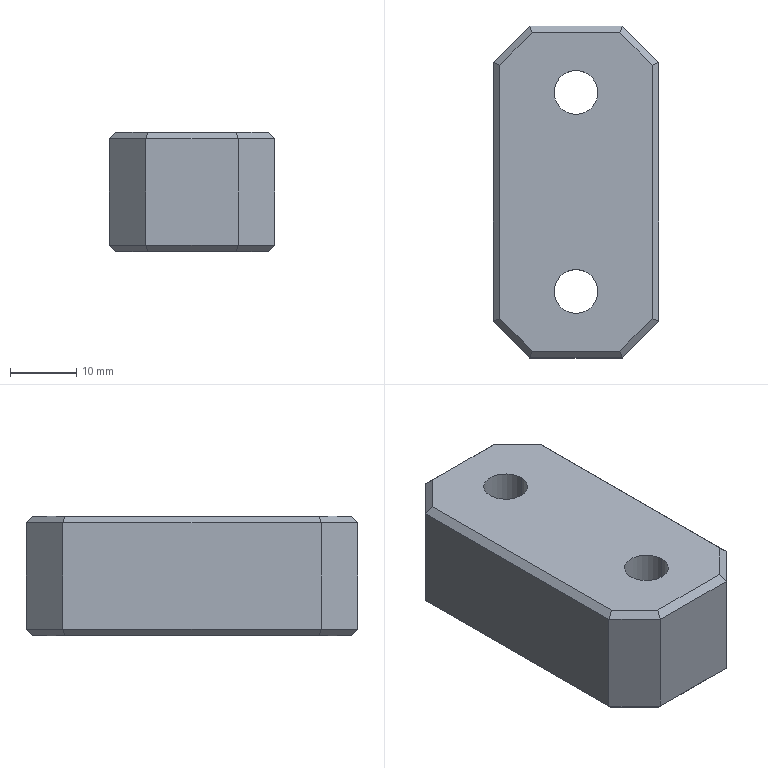Part | Creo | 1 solid | 36 faces | box 25 x 50 x 18 mm | volume 19193 mm3 | plane 28 | cylinder 8 | commonest cylinder face diameters 6.6 x4 11 x4
STEP:
#1=CARTESIAN_POINT('',(-67.892,-56.403,-348.));
#2=VERTEX_POINT('',#1);
#3=CARTESIAN_POINT('',(-54.721,-56.403,-348.));
#4=VERTEX_POINT('',#3);
#5=CARTESIAN_POINT('',(-67.892,-56.403,-348.));
#6=DIRECTION('',(1.,0.,0.));
#7=VECTOR('',#6,13.172);
#8=LINE('',#5,#7);
#9=EDGE_CURVE('',#2,#4,#8,.T.);
#10=ORIENTED_EDGE('',*,*,#9,.T.);
#11=CARTESIAN_POINT('',(-49.807,-61.317,-348.));
#12=VERTEX_POINT('',#11);
#13=CARTESIAN_POINT('',(-49.807,-61.317,-348.));
#14=DIRECTION('',(-0.7071,0.7071,0.));
#15=VECTOR('',#14,6.95);
#16=LINE('',#13,#15);
#17=EDGE_CURVE('',#12,#4,#16,.T.);
#18=ORIENTED_EDGE('',*,*,#17,.F.);
#19=CARTESIAN_POINT('',(-49.807,-99.489,-348.));
#20=VERTEX_POINT('',#19);
#21=CARTESIAN_POINT('',(-49.807,-99.489,-348.));
#22=DIRECTION('',(0.,1.,0.));
#23=VECTOR('',#22,38.172);
#24=LINE('',#21,#23);
#25=EDGE_CURVE('',#20,#12,#24,.T.);
#26=ORIENTED_EDGE('',*,*,#25,.F.);
#27=CARTESIAN_POINT('',(-54.721,-104.403,-348.));
#28=VERTEX_POINT('',#27);
#29=CARTESIAN_POINT('',(-54.721,-104.403,-348.));
#30=DIRECTION('',(0.7071,0.7071,0.));
#31=VECTOR('',#30,6.95);
#32=LINE('',#29,#31);
#33=EDGE_CURVE('',#28,#20,#32,.T.);
#34=ORIENTED_EDGE('',*,*,#33,.F.);
#35=CARTESIAN_POINT('',(-67.892,-104.403,-348.));
#36=VERTEX_POINT('',#35);
#37=CARTESIAN_POINT('',(-67.892,-104.403,-348.));
#38=DIRECTION('',(1.,0.,0.));
#39=VECTOR('',#38,13.172);
#40=LINE('',#37,#39);
#41=EDGE_CURVE('',#36,#28,#40,.T.);
#42=ORIENTED_EDGE('',*,*,#41,.F.);
#43=CARTESIAN_POINT('',(-72.807,-99.489,-348.));
#44=VERTEX_POINT('',#43);
#45=CARTESIAN_POINT('',(-72.807,-99.489,-348.));
#46=DIRECTION('',(0.7071,-0.7071,0.));
#47=VECTOR('',#46,6.95);
#48=LINE('',#45,#47);
#49=EDGE_CURVE('',#44,#36,#48,.T.);
#50=ORIENTED_EDGE('',*,*,#49,.F.);
#51=CARTESIAN_POINT('',(-72.807,-61.317,-348.));
#52=VERTEX_POINT('',#51);
#53=CARTESIAN_POINT('',(-72.807,-61.317,-348.));
#54=DIRECTION('',(0.,-1.,0.));
#55=VECTOR('',#54,38.172);
#56=LINE('',#53,#55);
#57=EDGE_CURVE('',#52,#44,#56,.T.);
#58=ORIENTED_EDGE('',*,*,#57,.F.);
#59=CARTESIAN_POINT('',(-67.892,-56.403,-348.));
#60=DIRECTION('',(-0.7071,-0.7071,0.));
#61=VECTOR('',#60,6.95);
#62=LINE('',#59,#61);
#63=EDGE_CURVE('',#2,#52,#62,.T.);
#64=ORIENTED_EDGE('',*,*,#63,.F.);
#65=EDGE_LOOP('',(#10,#18,#26,#34,#42,#50,#58,#64));
#66=FACE_OUTER_BOUND('',#65,.F.);
#67=CARTESIAN_POINT('',(-64.607,-95.403,-348.));
#68=VERTEX_POINT('',#67);
#69=CARTESIAN_POINT('',(-58.007,-95.403,-348.));
#70=VERTEX_POINT('',#69);
#71=CARTESIAN_POINT('',(-61.307,-95.403,-348.));
#72=DIRECTION('',(0.,0.,-1.));
#73=DIRECTION('',(-1.,0.,0.));
#74=AXIS2_PLACEMENT_3D('',#71,#72,#73);
#75=CIRCLE('',#74,3.3);
#76=EDGE_CURVE('',#68,#70,#75,.T.);
#77=ORIENTED_EDGE('',*,*,#76,.F.);
#78=CARTESIAN_POINT('',(-61.307,-95.403,-348.));
#79=DIRECTION('',(0.,0.,-1.));
#80=DIRECTION('',(1.,0.,0.));
#81=AXIS2_PLACEMENT_3D('',#78,#79,#80);
#82=CIRCLE('',#81,3.3);
#83=EDGE_CURVE('',#70,#68,#82,.T.);
#84=ORIENTED_EDGE('',*,*,#83,.F.);
#85=EDGE_LOOP('',(#77,#84));
#86=FACE_BOUND('',#85,.F.);
#87=CARTESIAN_POINT('',(-64.607,-65.403,-348.));
#88=VERTEX_POINT('',#87);
#89=CARTESIAN_POINT('',(-58.007,-65.403,-348.));
#90=VERTEX_POINT('',#89);
#91=CARTESIAN_POINT('',(-61.307,-65.403,-348.));
#92=DIRECTION('',(0.,0.,-1.));
#93=DIRECTION('',(-1.,0.,0.));
#94=AXIS2_PLACEMENT_3D('',#91,#92,#93);
#95=CIRCLE('',#94,3.3);
#96=EDGE_CURVE('',#88,#90,#95,.T.);
#97=ORIENTED_EDGE('',*,*,#96,.F.);
#98=CARTESIAN_POINT('',(-61.307,-65.403,-348.));
#99=DIRECTION('',(0.,0.,-1.));
#100=DIRECTION('',(1.,0.,0.));
#101=AXIS2_PLACEMENT_3D('',#98,#99,#100);
#102=CIRCLE('',#101,3.3);
#103=EDGE_CURVE('',#90,#88,#102,.T.);
#104=ORIENTED_EDGE('',*,*,#103,.F.);
#105=EDGE_LOOP('',(#97,#104));
#106=FACE_BOUND('',#105,.F.);
#107=CARTESIAN_POINT('',(-61.307,-75.403,-348.));
#108=DIRECTION('',(0.,0.,1.));
#109=DIRECTION('',(0.,1.,0.));
#110=AXIS2_PLACEMENT_3D('',#107,#108,#109);
#111=PLANE('',#110);
#112=ADVANCED_FACE('',(#66,#86,#106),#111,.T.);
#113=ORIENTED_EDGE('',*,*,#76,.T.);
#114=CARTESIAN_POINT('',(-58.007,-95.403,-359.));
#115=VERTEX_POINT('',#114);
#116=CARTESIAN_POINT('',(-58.007,-95.403,-348.));
#117=DIRECTION('',(0.,0.,-1.));
#118=VECTOR('',#117,11.);
#119=LINE('',#116,#118);
#120=EDGE_CURVE('',#70,#115,#119,.T.);
#121=ORIENTED_EDGE('',*,*,#120,.T.);
#122=CARTESIAN_POINT('',(-64.607,-95.403,-359.));
#123=VERTEX_POINT('',#122);
#124=CARTESIAN_POINT('',(-61.307,-95.403,-359.));
#125=DIRECTION('',(0.,0.,1.));
#126=DIRECTION('',(1.,0.,0.));
#127=AXIS2_PLACEMENT_3D('',#124,#125,#126);
#128=CIRCLE('',#127,3.3);
#129=EDGE_CURVE('',#115,#123,#128,.T.);
#130=ORIENTED_EDGE('',*,*,#129,.T.);
#131=CARTESIAN_POINT('',(-64.607,-95.403,-348.));
#132=DIRECTION('',(0.,0.,-1.));
#133=VECTOR('',#132,11.);
#134=LINE('',#131,#133);
#135=EDGE_CURVE('',#68,#123,#134,.T.);
#136=ORIENTED_EDGE('',*,*,#135,.F.);
#137=EDGE_LOOP('',(#113,#121,#130,#136));
#138=FACE_OUTER_BOUND('',#137,.F.);
#139=CARTESIAN_POINT('',(-61.307,-95.403,-366.));
#140=DIRECTION('',(0.,0.,-1.));
#141=DIRECTION('',(-1.,0.,0.));
#142=AXIS2_PLACEMENT_3D('',#139,#140,#141);
#143=CYLINDRICAL_SURFACE('',#142,3.3);
#144=ADVANCED_FACE('',(#138),#143,.F.);
#145=ORIENTED_EDGE('',*,*,#83,.T.);
#146=ORIENTED_EDGE('',*,*,#135,.T.);
#147=CARTESIAN_POINT('',(-61.307,-95.403,-359.));
#148=DIRECTION('',(0.,0.,1.));
#149=DIRECTION('',(-1.,0.,0.));
#150=AXIS2_PLACEMENT_3D('',#147,#148,#149);
#151=CIRCLE('',#150,3.3);
#152=EDGE_CURVE('',#123,#115,#151,.T.);
#153=ORIENTED_EDGE('',*,*,#152,.T.);
#154=ORIENTED_EDGE('',*,*,#120,.F.);
#155=EDGE_LOOP('',(#145,#146,#153,#154));
#156=FACE_OUTER_BOUND('',#155,.F.);
#157=CARTESIAN_POINT('',(-61.307,-95.403,-366.));
#158=DIRECTION('',(0.,0.,-1.));
#159=DIRECTION('',(-1.,0.,0.));
#160=AXIS2_PLACEMENT_3D('',#157,#158,#159);
#161=CYLINDRICAL_SURFACE('',#160,3.3);
#162=ADVANCED_FACE('',(#156),#161,.F.);
#163=CARTESIAN_POINT('',(-61.307,-89.903,-359.));
#164=VERTEX_POINT('',#163);
#165=CARTESIAN_POINT('',(-61.307,-100.903,-359.));
#166=VERTEX_POINT('',#165);
#167=CARTESIAN_POINT('',(-61.307,-95.403,-359.));
#168=DIRECTION('',(0.,0.,-1.));
#169=DIRECTION('',(0.,1.,0.));
#170=AXIS2_PLACEMENT_3D('',#167,#168,#169);
#171=CIRCLE('',#170,5.5);
#172=EDGE_CURVE('',#164,#166,#171,.T.);
#173=ORIENTED_EDGE('',*,*,#172,.F.);
#174=CARTESIAN_POINT('',(-61.307,-95.403,-359.));
#175=DIRECTION('',(0.,0.,-1.));
#176=DIRECTION('',(0.,-1.,0.));
#177=AXIS2_PLACEMENT_3D('',#174,#175,#176);
#178=CIRCLE('',#177,5.5);
#179=EDGE_CURVE('',#166,#164,#178,.T.);
#180=ORIENTED_EDGE('',*,*,#179,.F.);
#181=EDGE_LOOP('',(#173,#180));
#182=FACE_OUTER_BOUND('',#181,.F.);
#183=ORIENTED_EDGE('',*,*,#152,.F.);
#184=ORIENTED_EDGE('',*,*,#129,.F.);
#185=EDGE_LOOP('',(#183,#184));
#186=FACE_BOUND('',#185,.F.);
#187=CARTESIAN_POINT('',(-61.307,-95.403,-359.));
#188=DIRECTION('',(0.,0.,1.));
#189=DIRECTION('',(0.,1.,0.));
#190=AXIS2_PLACEMENT_3D('',#187,#188,#189);
#191=PLANE('',#190);
#192=ADVANCED_FACE('',(#182,#186),#191,.F.);
#193=ORIENTED_EDGE('',*,*,#172,.T.);
#194=CARTESIAN_POINT('',(-61.307,-100.903,-366.));
#195=VERTEX_POINT('',#194);
#196=CARTESIAN_POINT('',(-61.307,-100.903,-366.));
#197=DIRECTION('',(0.,0.,1.));
#198=VECTOR('',#197,7.);
#199=LINE('',#196,#198);
#200=EDGE_CURVE('',#195,#166,#199,.T.);
#201=ORIENTED_EDGE('',*,*,#200,.F.);
#202=CARTESIAN_POINT('',(-61.307,-89.903,-366.));
#203=VERTEX_POINT('',#202);
#204=CARTESIAN_POINT('',(-61.307,-95.403,-366.));
#205=DIRECTION('',(0.,0.,1.));
#206=DIRECTION('',(0.,-1.,0.));
#207=AXIS2_PLACEMENT_3D('',#204,#205,#206);
#208=CIRCLE('',#207,5.5);
#209=EDGE_CURVE('',#195,#203,#208,.T.);
#210=ORIENTED_EDGE('',*,*,#209,.T.);
#211=CARTESIAN_POINT('',(-61.307,-89.903,-366.));
#212=DIRECTION('',(0.,0.,1.));
#213=VECTOR('',#212,7.);
#214=LINE('',#211,#213);
#215=EDGE_CURVE('',#203,#164,#214,.T.);
#216=ORIENTED_EDGE('',*,*,#215,.T.);
#217=EDGE_LOOP('',(#193,#201,#210,#216));
#218=FACE_OUTER_BOUND('',#217,.F.);
#219=CARTESIAN_POINT('',(-61.307,-95.403,-372.));
#220=DIRECTION('',(0.,0.,1.));
#221=DIRECTION('',(0.,1.,0.));
#222=AXIS2_PLACEMENT_3D('',#219,#220,#221);
#223=CYLINDRICAL_SURFACE('',#222,5.5);
#224=ADVANCED_FACE('',(#218),#223,.F.);
#225=ORIENTED_EDGE('',*,*,#179,.T.);
#226=ORIENTED_EDGE('',*,*,#215,.F.);
#227=CARTESIAN_POINT('',(-61.307,-95.403,-366.));
#228=DIRECTION('',(0.,0.,1.));
#229=DIRECTION('',(0.,1.,0.));
#230=AXIS2_PLACEMENT_3D('',#227,#228,#229);
#231=CIRCLE('',#230,5.5);
#232=EDGE_CURVE('',#203,#195,#231,.T.);
#233=ORIENTED_EDGE('',*,*,#232,.T.);
#234=ORIENTED_EDGE('',*,*,#200,.T.);
#235=EDGE_LOOP('',(#225,#226,#233,#234));
#236=FACE_OUTER_BOUND('',#235,.F.);
#237=CARTESIAN_POINT('',(-61.307,-95.403,-372.));
#238=DIRECTION('',(0.,0.,1.));
#239=DIRECTION('',(0.,1.,0.));
#240=AXIS2_PLACEMENT_3D('',#237,#238,#239);
#241=CYLINDRICAL_SURFACE('',#240,5.5);
#242=ADVANCED_FACE('',(#236),#241,.F.);
#243=CARTESIAN_POINT('',(-49.807,-99.489,-366.));
#244=VERTEX_POINT('',#243);
#245=CARTESIAN_POINT('',(-54.721,-104.403,-366.));
#246=VERTEX_POINT('',#245);
#247=CARTESIAN_POINT('',(-49.807,-99.489,-366.));
#248=DIRECTION('',(-0.7071,-0.7071,0.));
#249=VECTOR('',#248,6.95);
#250=LINE('',#247,#249);
#251=EDGE_CURVE('',#244,#246,#250,.T.);
#252=ORIENTED_EDGE('',*,*,#251,.F.);
#253=CARTESIAN_POINT('',(-49.807,-61.317,-366.));
#254=VERTEX_POINT('',#253);
#255=CARTESIAN_POINT('',(-49.807,-61.317,-366.));
#256=DIRECTION('',(0.,-1.,0.));
#257=VECTOR('',#256,38.172);
#258=LINE('',#255,#257);
#259=EDGE_CURVE('',#254,#244,#258,.T.);
#260=ORIENTED_EDGE('',*,*,#259,.F.);
#261=CARTESIAN_POINT('',(-54.721,-56.403,-366.));
#262=VERTEX_POINT('',#261);
#263=CARTESIAN_POINT('',(-54.721,-56.403,-366.));
#264=DIRECTION('',(0.7071,-0.7071,0.));
#265=VECTOR('',#264,6.95);
#266=LINE('',#263,#265);
#267=EDGE_CURVE('',#262,#254,#266,.T.);
#268=ORIENTED_EDGE('',*,*,#267,.F.);
#269=CARTESIAN_POINT('',(-67.892,-56.403,-366.));
#270=VERTEX_POINT('',#269);
#271=CARTESIAN_POINT('',(-67.892,-56.403,-366.));
#272=DIRECTION('',(1.,0.,0.));
#273=VECTOR('',#272,13.172);
#274=LINE('',#271,#273);
#275=EDGE_CURVE('',#270,#262,#274,.T.);
#276=ORIENTED_EDGE('',*,*,#275,.F.);
#277=CARTESIAN_POINT('',(-72.807,-61.317,-366.));
#278=VERTEX_POINT('',#277);
#279=CARTESIAN_POINT('',(-72.807,-61.317,-366.));
#280=DIRECTION('',(0.7071,0.7071,0.));
#281=VECTOR('',#280,6.95);
#282=LINE('',#279,#281);
#283=EDGE_CURVE('',#278,#270,#282,.T.);
#284=ORIENTED_EDGE('',*,*,#283,.F.);
#285=CARTESIAN_POINT('',(-72.807,-99.489,-366.));
#286=VERTEX_POINT('',#285);
#287=CARTESIAN_POINT('',(-72.807,-99.489,-366.));
#288=DIRECTION('',(0.,1.,0.));
#289=VECTOR('',#288,38.172);
#290=LINE('',#287,#289);
#291=EDGE_CURVE('',#286,#278,#290,.T.);
#292=ORIENTED_EDGE('',*,*,#291,.F.);
#293=CARTESIAN_POINT('',(-67.892,-104.403,-366.));
#294=VERTEX_POINT('',#293);
#295=CARTESIAN_POINT('',(-67.892,-104.403,-366.));
#296=DIRECTION('',(-0.7071,0.7071,0.));
#297=VECTOR('',#296,6.95);
#298=LINE('',#295,#297);
#299=EDGE_CURVE('',#294,#286,#298,.T.);
#300=ORIENTED_EDGE('',*,*,#299,.F.);
#301=CARTESIAN_POINT('',(-67.892,-104.403,-366.));
#302=DIRECTION('',(1.,0.,0.));
#303=VECTOR('',#302,13.172);
#304=LINE('',#301,#303);
#305=EDGE_CURVE('',#294,#246,#304,.T.);
#306=ORIENTED_EDGE('',*,*,#305,.T.);
#307=EDGE_LOOP('',(#252,#260,#268,#276,#284,#292,#300,#306));
#308=FACE_OUTER_BOUND('',#307,.F.);
#309=ORIENTED_EDGE('',*,*,#232,.F.);
#310=ORIENTED_EDGE('',*,*,#209,.F.);
#311=EDGE_LOOP('',(#309,#310));
#312=FACE_BOUND('',#311,.F.);
#313=CARTESIAN_POINT('',(-61.307,-59.903,-366.));
#314=VERTEX_POINT('',#313);
#315=CARTESIAN_POINT('',(-61.307,-70.903,-366.));
#316=VERTEX_POINT('',#315);
#317=CARTESIAN_POINT('',(-61.307,-65.403,-366.));
#318=DIRECTION('',(0.,0.,1.));
#319=DIRECTION('',(0.,1.,0.));
#320=AXIS2_PLACEMENT_3D('',#317,#318,#319);
#321=CIRCLE('',#320,5.5);
#322=EDGE_CURVE('',#314,#316,#321,.T.);
#323=ORIENTED_EDGE('',*,*,#322,.F.);
#324=CARTESIAN_POINT('',(-61.307,-65.403,-366.));
#325=DIRECTION('',(0.,0.,1.));
#326=DIRECTION('',(0.,-1.,0.));
#327=AXIS2_PLACEMENT_3D('',#324,#325,#326);
#328=CIRCLE('',#327,5.5);
#329=EDGE_CURVE('',#316,#314,#328,.T.);
#330=ORIENTED_EDGE('',*,*,#329,.F.);
#331=EDGE_LOOP('',(#323,#330));
#332=FACE_BOUND('',#331,.F.);
#333=CARTESIAN_POINT('',(-61.307,-75.403,-366.));
#334=DIRECTION('',(0.,0.,1.));
#335=DIRECTION('',(0.,1.,0.));
#336=AXIS2_PLACEMENT_3D('',#333,#334,#335);
#337=PLANE('',#336);
#338=ADVANCED_FACE('',(#308,#312,#332),#337,.F.);
#339=CARTESIAN_POINT('',(-61.307,-70.903,-359.));
#340=VERTEX_POINT('',#339);
#341=CARTESIAN_POINT('',(-61.307,-59.903,-359.));
#342=VERTEX_POINT('',#341);
#343=CARTESIAN_POINT('',(-61.307,-65.403,-359.));
#344=DIRECTION('',(0.,0.,-1.));
#345=DIRECTION('',(0.,-1.,0.));
#346=AXIS2_PLACEMENT_3D('',#343,#344,#345);
#347=CIRCLE('',#346,5.5);
#348=EDGE_CURVE('',#340,#342,#347,.T.);
#349=ORIENTED_EDGE('',*,*,#348,.T.);
#350=CARTESIAN_POINT('',(-61.307,-59.903,-366.));
#351=DIRECTION('',(0.,0.,1.));
#352=VECTOR('',#351,7.);
#353=LINE('',#350,#352);
#354=EDGE_CURVE('',#314,#342,#353,.T.);
#355=ORIENTED_EDGE('',*,*,#354,.F.);
#356=ORIENTED_EDGE('',*,*,#322,.T.);
#357=CARTESIAN_POINT('',(-61.307,-70.903,-366.));
#358=DIRECTION('',(0.,0.,1.));
#359=VECTOR('',#358,7.);
#360=LINE('',#357,#359);
#361=EDGE_CURVE('',#316,#340,#360,.T.);
#362=ORIENTED_EDGE('',*,*,#361,.T.);
#363=EDGE_LOOP('',(#349,#355,#356,#362));
#364=FACE_OUTER_BOUND('',#363,.F.);
#365=CARTESIAN_POINT('',(-61.307,-65.403,-372.));
#366=DIRECTION('',(0.,0.,1.));
#367=DIRECTION('',(0.,1.,0.));
#368=AXIS2_PLACEMENT_3D('',#365,#366,#367);
#369=CYLINDRICAL_SURFACE('',#368,5.5);
#370=ADVANCED_FACE('',(#364),#369,.F.);
#371=CARTESIAN_POINT('',(-61.307,-65.403,-359.));
#372=DIRECTION('',(0.,0.,-1.));
#373=DIRECTION('',(0.,1.,0.));
#374=AXIS2_PLACEMENT_3D('',#371,#372,#373);
#375=CIRCLE('',#374,5.5);
#376=EDGE_CURVE('',#342,#340,#375,.T.);
#377=ORIENTED_EDGE('',*,*,#376,.F.);
#378=ORIENTED_EDGE('',*,*,#348,.F.);
#379=EDGE_LOOP('',(#377,#378));
#380=FACE_OUTER_BOUND('',#379,.F.);
#381=CARTESIAN_POINT('',(-64.607,-65.403,-359.));
#382=VERTEX_POINT('',#381);
#383=CARTESIAN_POINT('',(-58.007,-65.403,-359.));
#384=VERTEX_POINT('',#383);
#385=CARTESIAN_POINT('',(-61.307,-65.403,-359.));
#386=DIRECTION('',(0.,0.,1.));
#387=DIRECTION('',(-1.,0.,0.));
#388=AXIS2_PLACEMENT_3D('',#385,#386,#387);
#389=CIRCLE('',#388,3.3);
#390=EDGE_CURVE('',#382,#384,#389,.T.);
#391=ORIENTED_EDGE('',*,*,#390,.F.);
#392=CARTESIAN_POINT('',(-61.307,-65.403,-359.));
#393=DIRECTION('',(0.,0.,1.));
#394=DIRECTION('',(1.,0.,0.));
#395=AXIS2_PLACEMENT_3D('',#392,#393,#394);
#396=CIRCLE('',#395,3.3);
#397=EDGE_CURVE('',#384,#382,#396,.T.);
#398=ORIENTED_EDGE('',*,*,#397,.F.);
#399=EDGE_LOOP('',(#391,#398));
#400=FACE_BOUND('',#399,.F.);
#401=CARTESIAN_POINT('',(-61.307,-65.403,-359.));
#402=DIRECTION('',(0.,0.,1.));
#403=DIRECTION('',(0.,1.,0.));
#404=AXIS2_PLACEMENT_3D('',#401,#402,#403);
#405=PLANE('',#404);
#406=ADVANCED_FACE('',(#380,#400),#405,.F.);
#407=ORIENTED_EDGE('',*,*,#376,.T.);
#408=ORIENTED_EDGE('',*,*,#361,.F.);
#409=ORIENTED_EDGE('',*,*,#329,.T.);
#410=ORIENTED_EDGE('',*,*,#354,.T.);
#411=EDGE_LOOP('',(#407,#408,#409,#410));
#412=FACE_OUTER_BOUND('',#411,.F.);
#413=CARTESIAN_POINT('',(-61.307,-65.403,-372.));
#414=DIRECTION('',(0.,0.,1.));
#415=DIRECTION('',(0.,1.,0.));
#416=AXIS2_PLACEMENT_3D('',#413,#414,#415);
#417=CYLINDRICAL_SURFACE('',#416,5.5);
#418=ADVANCED_FACE('',(#412),#417,.F.);
#419=ORIENTED_EDGE('',*,*,#103,.T.);
#420=CARTESIAN_POINT('',(-64.607,-65.403,-348.));
#421=DIRECTION('',(0.,0.,-1.));
#422=VECTOR('',#421,11.);
#423=LINE('',#420,#422);
#424=EDGE_CURVE('',#88,#382,#423,.T.);
#425=ORIENTED_EDGE('',*,*,#424,.T.);
#426=ORIENTED_EDGE('',*,*,#390,.T.);
#427=CARTESIAN_POINT('',(-58.007,-65.403,-348.));
#428=DIRECTION('',(0.,0.,-1.));
#429=VECTOR('',#428,11.);
#430=LINE('',#427,#429);
#431=EDGE_CURVE('',#90,#384,#430,.T.);
#432=ORIENTED_EDGE('',*,*,#431,.F.);
#433=EDGE_LOOP('',(#419,#425,#426,#432));
#434=FACE_OUTER_BOUND('',#433,.F.);
#435=CARTESIAN_POINT('',(-61.307,-65.403,-366.));
#436=DIRECTION('',(0.,0.,-1.));
#437=DIRECTION('',(-1.,0.,0.));
#438=AXIS2_PLACEMENT_3D('',#435,#436,#437);
#439=CYLINDRICAL_SURFACE('',#438,3.3);
#440=ADVANCED_FACE('',(#434),#439,.F.);
#441=ORIENTED_EDGE('',*,*,#96,.T.);
#442=ORIENTED_EDGE('',*,*,#431,.T.);
#443=ORIENTED_EDGE('',*,*,#397,.T.);
#444=ORIENTED_EDGE('',*,*,#424,.F.);
#445=EDGE_LOOP('',(#441,#442,#443,#444));
#446=FACE_OUTER_BOUND('',#445,.F.);
#447=CARTESIAN_POINT('',(-61.307,-65.403,-366.));
#448=DIRECTION('',(0.,0.,-1.));
#449=DIRECTION('',(-1.,0.,0.));
#450=AXIS2_PLACEMENT_3D('',#447,#448,#449);
#451=CYLINDRICAL_SURFACE('',#450,3.3);
#452=ADVANCED_FACE('',(#446),#451,.F.);
#453=CARTESIAN_POINT('',(-48.807,-99.903,-365.));
#454=VERTEX_POINT('',#453);
#455=CARTESIAN_POINT('',(-54.307,-105.403,-365.));
#456=VERTEX_POINT('',#455);
#457=CARTESIAN_POINT('',(-48.807,-99.903,-365.));
#458=DIRECTION('',(-0.7071,-0.7071,0.));
#459=VECTOR('',#458,7.778);
#460=LINE('',#457,#459);
#461=EDGE_CURVE('',#454,#456,#460,.T.);
#462=ORIENTED_EDGE('',*,*,#461,.F.);
#463=CARTESIAN_POINT('',(-49.807,-99.489,-366.));
#464=DIRECTION('',(0.6786,-0.2811,0.6786));
#465=VECTOR('',#464,1.474);
#466=LINE('',#463,#465);
#467=EDGE_CURVE('',#244,#454,#466,.T.);
#468=ORIENTED_EDGE('',*,*,#467,.F.);
#469=ORIENTED_EDGE('',*,*,#251,.T.);
#470=CARTESIAN_POINT('',(-54.721,-104.403,-366.));
#471=DIRECTION('',(0.2811,-0.6786,0.6786));
#472=VECTOR('',#471,1.474);
#473=LINE('',#470,#472);
#474=EDGE_CURVE('',#246,#456,#473,.T.);
#475=ORIENTED_EDGE('',*,*,#474,.T.);
#476=EDGE_LOOP('',(#462,#468,#469,#475));
#477=FACE_OUTER_BOUND('',#476,.F.);
#478=CARTESIAN_POINT('',(-51.91,-102.299,-365.5));
#479=DIRECTION('',(0.5,-0.5,-0.7071));
#480=DIRECTION('',(0.5,-0.5,0.7071));
#481=AXIS2_PLACEMENT_3D('',#478,#479,#480);
#482=PLANE('',#481);
#483=ADVANCED_FACE('',(#477),#482,.T.);
#484=CARTESIAN_POINT('',(-54.307,-105.403,-349.));
#485=VERTEX_POINT('',#484);
#486=CARTESIAN_POINT('',(-54.307,-105.403,-365.));
#487=DIRECTION('',(0.,0.,1.));
#488=VECTOR('',#487,16.);
#489=LINE('',#486,#488);
#490=EDGE_CURVE('',#456,#485,#489,.T.);
#491=ORIENTED_EDGE('',*,*,#490,.T.);
#492=CARTESIAN_POINT('',(-48.807,-99.903,-349.));
#493=VERTEX_POINT('',#492);
#494=CARTESIAN_POINT('',(-54.307,-105.403,-349.));
#495=DIRECTION('',(0.7071,0.7071,0.));
#496=VECTOR('',#495,7.778);
#497=LINE('',#494,#496);
#498=EDGE_CURVE('',#485,#493,#497,.T.);
#499=ORIENTED_EDGE('',*,*,#498,.T.);
#500=CARTESIAN_POINT('',(-48.807,-99.903,-365.));
#501=DIRECTION('',(0.,0.,1.));
#502=VECTOR('',#501,16.);
#503=LINE('',#500,#502);
#504=EDGE_CURVE('',#454,#493,#503,.T.);
#505=ORIENTED_EDGE('',*,*,#504,.F.);
#506=ORIENTED_EDGE('',*,*,#461,.T.);
#507=EDGE_LOOP('',(#491,#499,#505,#506));
#508=FACE_OUTER_BOUND('',#507,.F.);
#509=CARTESIAN_POINT('',(-51.557,-102.653,-351.));
#510=DIRECTION('',(0.7071,-0.7071,0.));
#511=DIRECTION('',(0.7071,0.7071,0.));
#512=AXIS2_PLACEMENT_3D('',#509,#510,#511);
#513=PLANE('',#512);
#514=ADVANCED_FACE('',(#508),#513,.T.);
#515=CARTESIAN_POINT('',(-68.307,-105.403,-365.));
#516=VERTEX_POINT('',#515);
#517=CARTESIAN_POINT('',(-68.307,-105.403,-349.));
#518=VERTEX_POINT('',#517);
#519=CARTESIAN_POINT('',(-68.307,-105.403,-365.));
#520=DIRECTION('',(0.,0.,1.));
#521=VECTOR('',#520,16.);
#522=LINE('',#519,#521);
#523=EDGE_CURVE('',#516,#518,#522,.T.);
#524=ORIENTED_EDGE('',*,*,#523,.T.);
#525=CARTESIAN_POINT('',(-68.307,-105.403,-349.));
#526=DIRECTION('',(1.,0.,0.));
#527=VECTOR('',#526,14.);
#528=LINE('',#525,#527);
#529=EDGE_CURVE('',#518,#485,#528,.T.);
#530=ORIENTED_EDGE('',*,*,#529,.T.);
#531=ORIENTED_EDGE('',*,*,#490,.F.);
#532=CARTESIAN_POINT('',(-54.307,-105.403,-365.));
#533=DIRECTION('',(-1.,0.,0.));
#534=VECTOR('',#533,14.);
#535=LINE('',#532,#534);
#536=EDGE_CURVE('',#456,#516,#535,.T.);
#537=ORIENTED_EDGE('',*,*,#536,.T.);
#538=EDGE_LOOP('',(#524,#530,#531,#537));
#539=FACE_OUTER_BOUND('',#538,.F.);
#540=CARTESIAN_POINT('',(-46.307,-105.403,-354.));
#541=DIRECTION('',(0.,-1.,0.));
#542=DIRECTION('',(-1.,0.,0.));
#543=AXIS2_PLACEMENT_3D('',#540,#541,#542);
#544=PLANE('',#543);
#545=ADVANCED_FACE('',(#539),#544,.T.);
#546=CARTESIAN_POINT('',(-73.807,-99.903,-365.));
#547=VERTEX_POINT('',#546);
#548=CARTESIAN_POINT('',(-73.807,-99.903,-349.));
#549=VERTEX_POINT('',#548);
#550=CARTESIAN_POINT('',(-73.807,-99.903,-365.));
#551=DIRECTION('',(0.,0.,1.));
#552=VECTOR('',#551,16.);
#553=LINE('',#550,#552);
#554=EDGE_CURVE('',#547,#549,#553,.T.);
#555=ORIENTED_EDGE('',*,*,#554,.T.);
#556=CARTESIAN_POINT('',(-73.807,-99.903,-349.));
#557=DIRECTION('',(0.7071,-0.7071,0.));
#558=VECTOR('',#557,7.778);
#559=LINE('',#556,#558);
#560=EDGE_CURVE('',#549,#518,#559,.T.);
#561=ORIENTED_EDGE('',*,*,#560,.T.);
#562=ORIENTED_EDGE('',*,*,#523,.F.);
#563=CARTESIAN_POINT('',(-68.307,-105.403,-365.));
#564=DIRECTION('',(-0.7071,0.7071,0.));
#565=VECTOR('',#564,7.778);
#566=LINE('',#563,#565);
#567=EDGE_CURVE('',#516,#547,#566,.T.);
#568=ORIENTED_EDGE('',*,*,#567,.T.);
#569=EDGE_LOOP('',(#555,#561,#562,#568));
#570=FACE_OUTER_BOUND('',#569,.F.);
#571=CARTESIAN_POINT('',(-71.057,-102.653,-351.));
#572=DIRECTION('',(-0.7071,-0.7071,0.));
#573=DIRECTION('',(0.7071,-0.7071,0.));
#574=AXIS2_PLACEMENT_3D('',#571,#572,#573);
#575=PLANE('',#574);
#576=ADVANCED_FACE('',(#570),#575,.T.);
#577=CARTESIAN_POINT('',(-73.807,-60.903,-365.));
#578=VERTEX_POINT('',#577);
#579=CARTESIAN_POINT('',(-73.807,-60.903,-349.));
#580=VERTEX_POINT('',#579);
#581=CARTESIAN_POINT('',(-73.807,-60.903,-365.));
#582=DIRECTION('',(0.,0.,1.));
#583=VECTOR('',#582,16.);
#584=LINE('',#581,#583);
#585=EDGE_CURVE('',#578,#580,#584,.T.);
#586=ORIENTED_EDGE('',*,*,#585,.T.);
#587=CARTESIAN_POINT('',(-73.807,-60.903,-349.));
#588=DIRECTION('',(0.,-1.,0.));
#589=VECTOR('',#588,39.);
#590=LINE('',#587,#589);
#591=EDGE_CURVE('',#580,#549,#590,.T.);
#592=ORIENTED_EDGE('',*,*,#591,.T.);
#593=ORIENTED_EDGE('',*,*,#554,.F.);
#594=CARTESIAN_POINT('',(-73.807,-99.903,-365.));
#595=DIRECTION('',(0.,1.,0.));
#596=VECTOR('',#595,39.);
#597=LINE('',#594,#596);
#598=EDGE_CURVE('',#547,#578,#597,.T.);
#599=ORIENTED_EDGE('',*,*,#598,.T.);
#600=EDGE_LOOP('',(#586,#592,#593,#599));
#601=FACE_OUTER_BOUND('',#600,.F.);
#602=CARTESIAN_POINT('',(-73.807,-105.403,-354.));
#603=DIRECTION('',(-1.,0.,0.));
#604=DIRECTION('',(0.,1.,0.));
#605=AXIS2_PLACEMENT_3D('',#602,#603,#604);
#606=PLANE('',#605);
#607=ADVANCED_FACE('',(#601),#606,.T.);
#608=ORIENTED_EDGE('',*,*,#585,.F.);
#609=CARTESIAN_POINT('',(-68.307,-55.403,-365.));
#610=VERTEX_POINT('',#609);
#611=CARTESIAN_POINT('',(-73.807,-60.903,-365.));
#612=DIRECTION('',(0.7071,0.7071,0.));
#613=VECTOR('',#612,7.778);
#614=LINE('',#611,#613);
#615=EDGE_CURVE('',#578,#610,#614,.T.);
#616=ORIENTED_EDGE('',*,*,#615,.T.);
#617=CARTESIAN_POINT('',(-68.307,-55.403,-349.));
#618=VERTEX_POINT('',#617);
#619=CARTESIAN_POINT('',(-68.307,-55.403,-365.));
#620=DIRECTION('',(0.,0.,1.));
#621=VECTOR('',#620,16.);
#622=LINE('',#619,#621);
#623=EDGE_CURVE('',#610,#618,#622,.T.);
#624=ORIENTED_EDGE('',*,*,#623,.T.);
#625=CARTESIAN_POINT('',(-68.307,-55.403,-349.));
#626=DIRECTION('',(-0.7071,-0.7071,0.));
#627=VECTOR('',#626,7.778);
#628=LINE('',#625,#627);
#629=EDGE_CURVE('',#618,#580,#628,.T.);
#630=ORIENTED_EDGE('',*,*,#629,.T.);
#631=EDGE_LOOP('',(#608,#616,#624,#630));
#632=FACE_OUTER_BOUND('',#631,.F.);
#633=CARTESIAN_POINT('',(-71.057,-58.153,-351.));
#634=DIRECTION('',(-0.7071,0.7071,0.));
#635=DIRECTION('',(-0.7071,-0.7071,0.));
#636=AXIS2_PLACEMENT_3D('',#633,#634,#635);
#637=PLANE('',#636);
#638=ADVANCED_FACE('',(#632),#637,.T.);
#639=CARTESIAN_POINT('',(-72.807,-61.317,-366.));
#640=DIRECTION('',(-0.6786,0.2811,0.6786));
#641=VECTOR('',#640,1.474);
#642=LINE('',#639,#641);
#643=EDGE_CURVE('',#278,#578,#642,.T.);
#644=ORIENTED_EDGE('',*,*,#643,.F.);
#645=ORIENTED_EDGE('',*,*,#283,.T.);
#646=CARTESIAN_POINT('',(-67.892,-56.403,-366.));
#647=DIRECTION('',(-0.2811,0.6786,0.6786));
#648=VECTOR('',#647,1.474);
#649=LINE('',#646,#648);
#650=EDGE_CURVE('',#270,#610,#649,.T.);
#651=ORIENTED_EDGE('',*,*,#650,.T.);
#652=ORIENTED_EDGE('',*,*,#615,.F.);
#653=EDGE_LOOP('',(#644,#645,#651,#652));
#654=FACE_OUTER_BOUND('',#653,.F.);
#655=CARTESIAN_POINT('',(-70.703,-58.506,-365.5));
#656=DIRECTION('',(-0.5,0.5,-0.7071));
#657=DIRECTION('',(-0.5,0.5,0.7071));
#658=AXIS2_PLACEMENT_3D('',#655,#656,#657);
#659=PLANE('',#658);
#660=ADVANCED_FACE('',(#654),#659,.T.);
#661=CARTESIAN_POINT('',(-72.807,-99.489,-366.));
#662=DIRECTION('',(-0.6786,-0.2811,0.6786));
#663=VECTOR('',#662,1.474);
#664=LINE('',#661,#663);
#665=EDGE_CURVE('',#286,#547,#664,.T.);
#666=ORIENTED_EDGE('',*,*,#665,.F.);
#667=ORIENTED_EDGE('',*,*,#291,.T.);
#668=ORIENTED_EDGE('',*,*,#643,.T.);
#669=ORIENTED_EDGE('',*,*,#598,.F.);
#670=EDGE_LOOP('',(#666,#667,#668,#669));
#671=FACE_OUTER_BOUND('',#670,.F.);
#672=CARTESIAN_POINT('',(-73.307,-75.403,-365.5));
#673=DIRECTION('',(-0.7071,0.,-0.7071));
#674=DIRECTION('',(-0.7071,0.,0.7071));
#675=AXIS2_PLACEMENT_3D('',#672,#673,#674);
#676=PLANE('',#675);
#677=ADVANCED_FACE('',(#671),#676,.T.);
#678=ORIENTED_EDGE('',*,*,#299,.T.);
#679=ORIENTED_EDGE('',*,*,#665,.T.);
#680=ORIENTED_EDGE('',*,*,#567,.F.);
#681=CARTESIAN_POINT('',(-68.307,-105.403,-365.));
#682=DIRECTION('',(0.2811,0.6786,-0.6786));
#683=VECTOR('',#682,1.474);
#684=LINE('',#681,#683);
#685=EDGE_CURVE('',#516,#294,#684,.T.);
#686=ORIENTED_EDGE('',*,*,#685,.T.);
#687=EDGE_LOOP('',(#678,#679,#680,#686));
#688=FACE_OUTER_BOUND('',#687,.F.);
#689=CARTESIAN_POINT('',(-70.703,-102.299,-365.5));
#690=DIRECTION('',(-0.5,-0.5,-0.7071));
#691=DIRECTION('',(-0.5,-0.5,0.7071));
#692=AXIS2_PLACEMENT_3D('',#689,#690,#691);
#693=PLANE('',#692);
#694=ADVANCED_FACE('',(#688),#693,.T.);
#695=ORIENTED_EDGE('',*,*,#685,.F.);
#696=ORIENTED_EDGE('',*,*,#536,.F.);
#697=ORIENTED_EDGE('',*,*,#474,.F.);
#698=ORIENTED_EDGE('',*,*,#305,.F.);
#699=EDGE_LOOP('',(#695,#696,#697,#698));
#700=FACE_OUTER_BOUND('',#699,.F.);
#701=CARTESIAN_POINT('',(-46.307,-105.403,-365.));
#702=DIRECTION('',(0.,-0.7071,-0.7071));
#703=DIRECTION('',(-1.,0.,0.));
#704=AXIS2_PLACEMENT_3D('',#701,#702,#703);
#705=PLANE('',#704);
#706=ADVANCED_FACE('',(#700),#705,.T.);
#707=ORIENTED_EDGE('',*,*,#650,.F.);
#708=ORIENTED_EDGE('',*,*,#275,.T.);
#709=CARTESIAN_POINT('',(-54.307,-55.403,-365.));
#710=VERTEX_POINT('',#709);
#711=CARTESIAN_POINT('',(-54.721,-56.403,-366.));
#712=DIRECTION('',(0.2811,0.6786,0.6786));
#713=VECTOR('',#712,1.474);
#714=LINE('',#711,#713);
#715=EDGE_CURVE('',#262,#710,#714,.T.);
#716=ORIENTED_EDGE('',*,*,#715,.T.);
#717=CARTESIAN_POINT('',(-68.307,-55.403,-365.));
#718=DIRECTION('',(1.,0.,0.));
#719=VECTOR('',#718,14.);
#720=LINE('',#717,#719);
#721=EDGE_CURVE('',#610,#710,#720,.T.);
#722=ORIENTED_EDGE('',*,*,#721,.F.);
#723=EDGE_LOOP('',(#707,#708,#716,#722));
#724=FACE_OUTER_BOUND('',#723,.F.);
#725=CARTESIAN_POINT('',(-61.307,-55.903,-365.5));
#726=DIRECTION('',(0.,0.7071,-0.7071));
#727=DIRECTION('',(0.,0.7071,0.7071));
#728=AXIS2_PLACEMENT_3D('',#725,#726,#727);
#729=PLANE('',#728);
#730=ADVANCED_FACE('',(#724),#729,.T.);
#731=CARTESIAN_POINT('',(-48.807,-60.903,-365.));
#732=VERTEX_POINT('',#731);
#733=CARTESIAN_POINT('',(-49.807,-61.317,-366.));
#734=DIRECTION('',(0.6786,0.2811,0.6786));
#735=VECTOR('',#734,1.474);
#736=LINE('',#733,#735);
#737=EDGE_CURVE('',#254,#732,#736,.T.);
#738=ORIENTED_EDGE('',*,*,#737,.T.);
#739=CARTESIAN_POINT('',(-54.307,-55.403,-365.));
#740=DIRECTION('',(0.7071,-0.7071,0.));
#741=VECTOR('',#740,7.778);
#742=LINE('',#739,#741);
#743=EDGE_CURVE('',#710,#732,#742,.T.);
#744=ORIENTED_EDGE('',*,*,#743,.F.);
#745=ORIENTED_EDGE('',*,*,#715,.F.);
#746=ORIENTED_EDGE('',*,*,#267,.T.);
#747=EDGE_LOOP('',(#738,#744,#745,#746));
#748=FACE_OUTER_BOUND('',#747,.F.);
#749=CARTESIAN_POINT('',(-51.91,-58.506,-365.5));
#750=DIRECTION('',(0.5,0.5,-0.7071));
#751=DIRECTION('',(0.5,0.5,0.7071));
#752=AXIS2_PLACEMENT_3D('',#749,#750,#751);
#753=PLANE('',#752);
#754=ADVANCED_FACE('',(#748),#753,.T.);
#755=ORIENTED_EDGE('',*,*,#737,.F.);
#756=ORIENTED_EDGE('',*,*,#259,.T.);
#757=ORIENTED_EDGE('',*,*,#467,.T.);
#758=CARTESIAN_POINT('',(-48.807,-60.903,-365.));
#759=DIRECTION('',(0.,-1.,0.));
#760=VECTOR('',#759,39.);
#761=LINE('',#758,#760);
#762=EDGE_CURVE('',#732,#454,#761,.T.);
#763=ORIENTED_EDGE('',*,*,#762,.F.);
#764=EDGE_LOOP('',(#755,#756,#757,#763));
#765=FACE_OUTER_BOUND('',#764,.F.);
#766=CARTESIAN_POINT('',(-49.307,-75.403,-365.5));
#767=DIRECTION('',(0.7071,0.,-0.7071));
#768=DIRECTION('',(0.7071,0.,0.7071));
#769=AXIS2_PLACEMENT_3D('',#766,#767,#768);
#770=PLANE('',#769);
#771=ADVANCED_FACE('',(#765),#770,.T.);
#772=ORIENTED_EDGE('',*,*,#504,.T.);
#773=CARTESIAN_POINT('',(-48.807,-60.903,-349.));
#774=VERTEX_POINT('',#773);
#775=CARTESIAN_POINT('',(-48.807,-99.903,-349.));
#776=DIRECTION('',(0.,1.,0.));
#777=VECTOR('',#776,39.);
#778=LINE('',#775,#777);
#779=EDGE_CURVE('',#493,#774,#778,.T.);
#780=ORIENTED_EDGE('',*,*,#779,.T.);
#781=CARTESIAN_POINT('',(-48.807,-60.903,-365.));
#782=DIRECTION('',(0.,0.,1.));
#783=VECTOR('',#782,16.);
#784=LINE('',#781,#783);
#785=EDGE_CURVE('',#732,#774,#784,.T.);
#786=ORIENTED_EDGE('',*,*,#785,.F.);
#787=ORIENTED_EDGE('',*,*,#762,.T.);
#788=EDGE_LOOP('',(#772,#780,#786,#787));
#789=FACE_OUTER_BOUND('',#788,.F.);
#790=CARTESIAN_POINT('',(-48.807,-45.403,-354.));
#791=DIRECTION('',(1.,0.,0.));
#792=DIRECTION('',(0.,-1.,0.));
#793=AXIS2_PLACEMENT_3D('',#790,#791,#792);
#794=PLANE('',#793);
#795=ADVANCED_FACE('',(#789),#794,.T.);
#796=ORIENTED_EDGE('',*,*,#779,.F.);
#797=CARTESIAN_POINT('',(-49.807,-99.489,-348.));
#798=DIRECTION('',(0.6786,-0.2811,-0.6786));
#799=VECTOR('',#798,1.474);
#800=LINE('',#797,#799);
#801=EDGE_CURVE('',#20,#493,#800,.T.);
#802=ORIENTED_EDGE('',*,*,#801,.F.);
#803=ORIENTED_EDGE('',*,*,#25,.T.);
#804=CARTESIAN_POINT('',(-49.807,-61.317,-348.));
#805=DIRECTION('',(0.6786,0.2811,-0.6786));
#806=VECTOR('',#805,1.474);
#807=LINE('',#804,#806);
#808=EDGE_CURVE('',#12,#774,#807,.T.);
#809=ORIENTED_EDGE('',*,*,#808,.T.);
#810=EDGE_LOOP('',(#796,#802,#803,#809));
#811=FACE_OUTER_BOUND('',#810,.F.);
#812=CARTESIAN_POINT('',(-49.307,-75.403,-348.5));
#813=DIRECTION('',(0.7071,0.,0.7071));
#814=DIRECTION('',(0.7071,0.,-0.7071));
#815=AXIS2_PLACEMENT_3D('',#812,#813,#814);
#816=PLANE('',#815);
#817=ADVANCED_FACE('',(#811),#816,.T.);
#818=CARTESIAN_POINT('',(-54.721,-104.403,-348.));
#819=DIRECTION('',(0.2811,-0.6786,-0.6786));
#820=VECTOR('',#819,1.474);
#821=LINE('',#818,#820);
#822=EDGE_CURVE('',#28,#485,#821,.T.);
#823=ORIENTED_EDGE('',*,*,#822,.F.);
#824=ORIENTED_EDGE('',*,*,#33,.T.);
#825=ORIENTED_EDGE('',*,*,#801,.T.);
#826=ORIENTED_EDGE('',*,*,#498,.F.);
#827=EDGE_LOOP('',(#823,#824,#825,#826));
#828=FACE_OUTER_BOUND('',#827,.F.);
#829=CARTESIAN_POINT('',(-51.91,-102.299,-348.5));
#830=DIRECTION('',(0.5,-0.5,0.7071));
#831=DIRECTION('',(0.5,-0.5,-0.7071));
#832=AXIS2_PLACEMENT_3D('',#829,#830,#831);
#833=PLANE('',#832);
#834=ADVANCED_FACE('',(#828),#833,.T.);
#835=CARTESIAN_POINT('',(-67.892,-104.403,-348.));
#836=DIRECTION('',(-0.2811,-0.6786,-0.6786));
#837=VECTOR('',#836,1.474);
#838=LINE('',#835,#837);
#839=EDGE_CURVE('',#36,#518,#838,.T.);
#840=ORIENTED_EDGE('',*,*,#839,.F.);
#841=ORIENTED_EDGE('',*,*,#41,.T.);
#842=ORIENTED_EDGE('',*,*,#822,.T.);
#843=ORIENTED_EDGE('',*,*,#529,.F.);
#844=EDGE_LOOP('',(#840,#841,#842,#843));
#845=FACE_OUTER_BOUND('',#844,.F.);
#846=CARTESIAN_POINT('',(-61.307,-104.903,-348.5));
#847=DIRECTION('',(0.,-0.7071,0.7071));
#848=DIRECTION('',(0.,-0.7071,-0.7071));
#849=AXIS2_PLACEMENT_3D('',#846,#847,#848);
#850=PLANE('',#849);
#851=ADVANCED_FACE('',(#845),#850,.T.);
#852=CARTESIAN_POINT('',(-72.807,-99.489,-348.));
#853=DIRECTION('',(-0.6786,-0.2811,-0.6786));
#854=VECTOR('',#853,1.474);
#855=LINE('',#852,#854);
#856=EDGE_CURVE('',#44,#549,#855,.T.);
#857=ORIENTED_EDGE('',*,*,#856,.F.);
#858=ORIENTED_EDGE('',*,*,#49,.T.);
#859=ORIENTED_EDGE('',*,*,#839,.T.);
#860=ORIENTED_EDGE('',*,*,#560,.F.);
#861=EDGE_LOOP('',(#857,#858,#859,#860));
#862=FACE_OUTER_BOUND('',#861,.F.);
#863=CARTESIAN_POINT('',(-70.703,-102.299,-348.5));
#864=DIRECTION('',(-0.5,-0.5,0.7071));
#865=DIRECTION('',(-0.5,-0.5,-0.7071));
#866=AXIS2_PLACEMENT_3D('',#863,#864,#865);
#867=PLANE('',#866);
#868=ADVANCED_FACE('',(#862),#867,.T.);
#869=ORIENTED_EDGE('',*,*,#57,.T.);
#870=ORIENTED_EDGE('',*,*,#856,.T.);
#871=ORIENTED_EDGE('',*,*,#591,.F.);
#872=CARTESIAN_POINT('',(-73.807,-60.903,-349.));
#873=DIRECTION('',(0.6786,-0.2811,0.6786));
#874=VECTOR('',#873,1.474);
#875=LINE('',#872,#874);
#876=EDGE_CURVE('',#580,#52,#875,.T.);
#877=ORIENTED_EDGE('',*,*,#876,.T.);
#878=EDGE_LOOP('',(#869,#870,#871,#877));
#879=FACE_OUTER_BOUND('',#878,.F.);
#880=CARTESIAN_POINT('',(-73.307,-75.403,-348.5));
#881=DIRECTION('',(-0.7071,0.,0.7071));
#882=DIRECTION('',(-0.7071,0.,-0.7071));
#883=AXIS2_PLACEMENT_3D('',#880,#881,#882);
#884=PLANE('',#883);
#885=ADVANCED_FACE('',(#879),#884,.T.);
#886=ORIENTED_EDGE('',*,*,#876,.F.);
#887=ORIENTED_EDGE('',*,*,#629,.F.);
#888=CARTESIAN_POINT('',(-68.307,-55.403,-349.));
#889=DIRECTION('',(0.2811,-0.6786,0.6786));
#890=VECTOR('',#889,1.474);
#891=LINE('',#888,#890);
#892=EDGE_CURVE('',#618,#2,#891,.T.);
#893=ORIENTED_EDGE('',*,*,#892,.T.);
#894=ORIENTED_EDGE('',*,*,#63,.T.);
#895=EDGE_LOOP('',(#886,#887,#893,#894));
#896=FACE_OUTER_BOUND('',#895,.F.);
#897=CARTESIAN_POINT('',(-71.057,-58.153,-349.));
#898=DIRECTION('',(0.5,-0.5,-0.7071));
#899=DIRECTION('',(0.7071,0.7071,0.));
#900=AXIS2_PLACEMENT_3D('',#897,#898,#899);
#901=PLANE('',#900);
#902=ADVANCED_FACE('',(#896),#901,.F.);
#903=CARTESIAN_POINT('',(-54.307,-55.403,-349.));
#904=VERTEX_POINT('',#903);
#905=CARTESIAN_POINT('',(-54.307,-55.403,-349.));
#906=DIRECTION('',(-0.2811,-0.6786,0.6786));
#907=VECTOR('',#906,1.474);
#908=LINE('',#905,#907);
#909=EDGE_CURVE('',#904,#4,#908,.T.);
#910=ORIENTED_EDGE('',*,*,#909,.T.);
#911=ORIENTED_EDGE('',*,*,#9,.F.);
#912=ORIENTED_EDGE('',*,*,#892,.F.);
#913=CARTESIAN_POINT('',(-54.307,-55.403,-349.));
#914=DIRECTION('',(-1.,0.,0.));
#915=VECTOR('',#914,14.);
#916=LINE('',#913,#915);
#917=EDGE_CURVE('',#904,#618,#916,.T.);
#918=ORIENTED_EDGE('',*,*,#917,.F.);
#919=EDGE_LOOP('',(#910,#911,#912,#918));
#920=FACE_OUTER_BOUND('',#919,.F.);
#921=CARTESIAN_POINT('',(-76.307,-55.403,-349.));
#922=DIRECTION('',(0.,-0.7071,-0.7071));
#923=DIRECTION('',(1.,0.,0.));
#924=AXIS2_PLACEMENT_3D('',#921,#922,#923);
#925=PLANE('',#924);
#926=ADVANCED_FACE('',(#920),#925,.F.);
#927=ORIENTED_EDGE('',*,*,#808,.F.);
#928=ORIENTED_EDGE('',*,*,#17,.T.);
#929=ORIENTED_EDGE('',*,*,#909,.F.);
#930=CARTESIAN_POINT('',(-48.807,-60.903,-349.));
#931=DIRECTION('',(-0.7071,0.7071,0.));
#932=VECTOR('',#931,7.778);
#933=LINE('',#930,#932);
#934=EDGE_CURVE('',#774,#904,#933,.T.);
#935=ORIENTED_EDGE('',*,*,#934,.F.);
#936=EDGE_LOOP('',(#927,#928,#929,#935));
#937=FACE_OUTER_BOUND('',#936,.F.);
#938=CARTESIAN_POINT('',(-51.557,-58.153,-349.));
#939=DIRECTION('',(-0.5,-0.5,-0.7071));
#940=DIRECTION('',(0.7071,-0.7071,0.));
#941=AXIS2_PLACEMENT_3D('',#938,#939,#940);
#942=PLANE('',#941);
#943=ADVANCED_FACE('',(#937),#942,.F.);
#944=CARTESIAN_POINT('',(-54.307,-55.403,-365.));
#945=DIRECTION('',(0.,0.,1.));
#946=VECTOR('',#945,16.);
#947=LINE('',#944,#946);
#948=EDGE_CURVE('',#710,#904,#947,.T.);
#949=ORIENTED_EDGE('',*,*,#948,.F.);
#950=ORIENTED_EDGE('',*,*,#743,.T.);
#951=ORIENTED_EDGE('',*,*,#785,.T.);
#952=ORIENTED_EDGE('',*,*,#934,.T.);
#953=EDGE_LOOP('',(#949,#950,#951,#952));
#954=FACE_OUTER_BOUND('',#953,.F.);
#955=CARTESIAN_POINT('',(-51.557,-58.153,-351.));
#956=DIRECTION('',(0.7071,0.7071,0.));
#957=DIRECTION('',(-0.7071,0.7071,0.));
#958=AXIS2_PLACEMENT_3D('',#955,#956,#957);
#959=PLANE('',#958);
#960=ADVANCED_FACE('',(#954),#959,.T.);
#961=ORIENTED_EDGE('',*,*,#623,.F.);
#962=ORIENTED_EDGE('',*,*,#721,.T.);
#963=ORIENTED_EDGE('',*,*,#948,.T.);
#964=ORIENTED_EDGE('',*,*,#917,.T.);
#965=EDGE_LOOP('',(#961,#962,#963,#964));
#966=FACE_OUTER_BOUND('',#965,.F.);
#967=CARTESIAN_POINT('',(-76.307,-55.403,-354.));
#968=DIRECTION('',(0.,1.,0.));
#969=DIRECTION('',(1.,0.,0.));
#970=AXIS2_PLACEMENT_3D('',#967,#968,#969);
#971=PLANE('',#970);
#972=ADVANCED_FACE('',(#966),#971,.T.);
#973=CLOSED_SHELL('',(#112,#144,#162,#192,#224,#242,#338,#370,#406,#418,#440,#452,#483,#514,#545,#576,#607,#638,#660,#677,#694,#706,#730,#754,#771,#795,#817,#834,#851,#868,#885,#902,#926,#943,#960,#972));
#974=MANIFOLD_SOLID_BREP('',#973);
#975=(LENGTH_UNIT()NAMED_UNIT(*)SI_UNIT(.MILLI.,.METRE.));
#976=UNCERTAINTY_MEASURE_WITH_UNIT(LENGTH_MEASURE(0.005873),#975,'','');
#977=(NAMED_UNIT(*)PLANE_ANGLE_UNIT()SI_UNIT($,.RADIAN.));
#978=PLANE_ANGLE_MEASURE_WITH_UNIT(PLANE_ANGLE_MEASURE(0.01745),#977);
#979=(CONVERSION_BASED_UNIT('DEGREE',#978)NAMED_UNIT(*)PLANE_ANGLE_UNIT());
#980=(NAMED_UNIT(*)SI_UNIT($,.STERADIAN.)SOLID_ANGLE_UNIT());
#981=(GEOMETRIC_REPRESENTATION_CONTEXT(3)GLOBAL_UNCERTAINTY_ASSIGNED_CONTEXT((#976))GLOBAL_UNIT_ASSIGNED_CONTEXT((#975,#979,#980))REPRESENTATION_CONTEXT('',''));
#982=ADVANCED_BREP_SHAPE_REPRESENTATION('',(#974),#981);